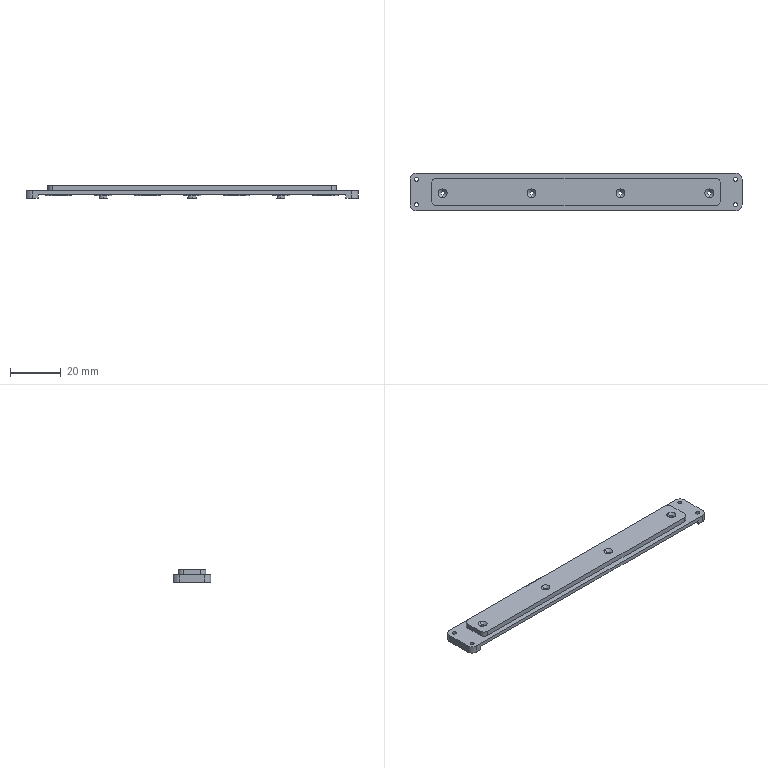NC program | NX | posted with a generic post | part box 130.666 x 14.95 x 5 mm
Lines 1 to 1700 of 3855:
N10 G17 G21 G94 G90
(FLOOR_WALL_COPY_COPY , TOOL : D80)
N12 T19 M6
N14 G54
N16 G17 G0 G90 X110.333 Y0. S6500 M3
N18 G43 Z30. H19
N20 Z5.5
N22 G94 G1 Z2.5 F1500.
N24 X105.333
N26 X-105.333
N28 X-110.333
N30 Z5.5
N32 G0 Z30.
N34 X110.333
N36 Z5.
N38 G1 Z2.
N40 X105.333
N42 X-105.333
N44 X-110.333
N46 Z5.
N48 G0 Z30.
N50 X110.333
N52 Z4.5
N54 G1 Z1.5
N56 X105.333
N58 X-105.333
N60 X-110.333
N62 Z4.5
N64 G0 Z30.
N66 X110.333
N68 Z4.
N70 G1 Z1.
N72 X105.333
N74 X-105.333
N76 X-110.333
N78 Z4.
N80 G0 Z30.
N82 X110.333
N84 Z3.5
N86 G1 Z0.5
N88 X105.333
N90 X-105.333
N92 X-110.333
N94 Z3.5
N96 G0 Z30.
N98 X110.333
N100 Z3.
N102 G1 Z0.
N104 X105.333
N106 X-105.333
N108 X-110.333
N110 Z3.
N112 G0 Z30.
N114 M5
(DRILLING_COPY_1_COPY_2 , TOOL : D6A45)
N116 T01 M6
N118 G54
N120 G17 G0 G90 X-34.994 Y0. S5000 M3
N122 G43 Z30. H1
N124 G94 G81 G98 Z-1.1 F350. R3.
N126 X0.006
N128 X35.006
N130 G80
N132 G0 X35.006 Y0. Z30.
N134 M5
(DRILLING_COPY_1_COPY_COPY_COPY , TOOL : 1.6ZT)
N136 T17 M6
N138 G54
N140 G17 G0 G90 X-34.994 Y0. S2000 M3
N142 G43 Z30. H17
N144 G94 G83 G98 Z-3.5 F100. Q2. R3.
N146 X35.006
N148 X0.006
N150 G80
N152 G0 X0.006 Y0. Z30.
N154 M5
(CAVITY_MILL , TOOL : D10)
N156 T15 M6
N158 G54
N160 G17 G0 G90 X-17.283 Y-14.473 S9500 M3
N162 G43 Z30. H15
N164 Z0.1
N166 G94 G1 Z-0.9 F1000.
N168 Y-8.02
N170 G3 X-17.494 Y-7.973 R0.5
N172 G1 Y-1.973
N174 X-7.644 F2500.
N176 G2 X-7.644 Y1.973 R7.9
N178 G1 X-6.482 Y1.673
N180 G2 X1.679 Y6.488 R6.7
N182 X-6.482 Y1.673 R-6.7
N184 G1 X-7.644 Y1.973
N186 X-27.345
N188 G2 X-27.345 Y-1.973 R7.9
N190 G1 X-28.507 Y-1.673
N192 G2 X-36.668 Y-6.488 R6.7
N194 X-28.507 Y-1.673 R-6.7
N196 G1 X-27.345 Y-1.973
N198 X-17.494
N200 Y-7.973
N202 X7.655
N204 Y-1.973
N206 X27.356
N208 G2 X27.356 Y1.973 R7.9
N210 G1 X28.518 Y1.673
N212 G2 X36.679 Y6.488 R6.7
N214 X28.518 Y1.673 R-6.7
N216 G1 X27.356 Y1.973
N218 X7.655
N220 G2 X7.655 Y-1.973 R7.9
N222 G1 Y-7.973
N224 X42.655
N226 Y-1.973
N228 X49.406
N230 Y1.973
N232 X42.655
N234 G2 X42.655 Y-1.973 R7.9
N236 G1 Y-7.973
N238 X54.225
N240 G3 X56.67 Y-12.473 R6.3
N242 G1 X59.491
N244 G2 X55.406 Y-7.475 R5.1
N246 G1 Y7.475
N248 G2 X59.491 Y12.473 R5.1
N250 G1 X56.67
N252 G3 X54.225 Y7.973 R6.3
N254 G1 X-42.644
N256 Y1.973
N258 X-49.394
N260 Y-1.973
N262 X-42.644
N264 G2 X-42.644 Y1.973 R7.9
N266 G1 Y7.973
N268 X-54.214
N270 G3 X-56.659 Y12.473 R6.3
N272 G1 X-59.479
N274 G2 X-55.394 Y7.475 R5.1
N276 G1 Y-7.475
N278 G2 X-59.479 Y-12.473 R5.1
N280 G1 X-56.659
N282 G3 X-54.214 Y-7.973 R6.3
N284 G1 X-17.494
N286 G2 X-16.728 Y-8.33 R1.
N288 G1 X-11.574 Y-14.473
N290 Z0.1
N292 G0 X-2.139 Z-0.4
N294 G1 Z-1.4 F1000.
N296 X-0.76 Y-12.83
N298 G2 X0.006 Y-12.473 R1.
N300 G1 X59.492 F2500.
N302 G2 X56.374 Y-10.464 R5.1
N304 X55.081 Y-10.575 R7.6
N306 G1 X49.931
N308 G2 X42.448 Y-4.31 R7.601
N310 X27.563 Y-4.309 R8.6
N312 X20.081 Y-10.575 R7.6
N314 G1 X14.931
N316 G2 X7.449 Y-4.309 R7.6
N318 X-7.437 Y-4.309 R8.6
N320 X-14.919 Y-10.575 R7.6
N322 G1 X-20.069
N324 G2 X-27.551 Y-4.309 R7.6
N326 X-42.437 Y-4.309 R8.6
N328 X-49.919 Y-10.575 R7.6
N330 G1 X-55.069
N332 G2 X-56.362 Y-10.464 R7.6
N334 X-59.481 Y-12.473 R5.1
N336 G1 X0.006
N338 G2 X0.772 Y-12.83 R1.
N340 G1 X2.15 Y-14.473
N342 Z-0.4
N344 G0 Z30.
N346 Y14.473
N348 Z-0.4
N350 G1 Z-1.4 F1000.
N352 X0.772 Y12.83
N354 G2 X0.006 Y12.473 R1.
N356 G1 X-59.481 F2500.
N358 G2 X-56.362 Y10.464 R5.1
N360 X-55.069 Y10.575 R7.6
N362 G1 X-49.919
N364 G2 X-42.436 Y4.31 R7.601
N366 X-27.551 Y4.309 R8.6
N368 X-20.069 Y10.575 R7.6
N370 G1 X-14.919
N372 G2 X-7.437 Y4.309 R7.6
N374 X7.449 Y4.309 R8.6
N376 X14.931 Y10.575 R7.6
N378 G1 X20.081
N380 G2 X27.563 Y4.309 R7.6
N382 X42.449 Y4.31 R8.601
N384 X49.931 Y10.575 R7.6
N386 G1 X55.081
N388 G2 X56.374 Y10.464 R7.6
N390 X59.492 Y12.473 R5.1
N392 G1 X0.006
N394 G2 X-0.76 Y12.83 R1.
N396 G1 X-2.139 Y14.473
N398 Z-0.4
N400 G0 Z30.
N402 M5
(CAVITY_MILL_COPY , TOOL : D4)
N404 T11 M6
N406 G54
N408 G17 G0 G90 X59.073 Y-9.881 S9500 M3
N410 G43 Z30. H11
N412 Z-0.25
N414 G94 G1 Z-1.25 F1000.
N416 X59.141 Y-9.544
N418 G3 X58.942 Y-8.722 R1.
N420 G2 X58.506 Y-7.475 R2. F1500.
N422 G1 Y-5.894
N424 G2 X55.851 Y-7.409 R4.5
N426 G3 X55.157 Y-7.892 R1.
N428 G1 X54.935 Y-8.275
N430 Z-0.25
N432 G0 X59.073 Y-9.881 Z-0.5
N434 G1 Z-1.5 F1000.
N436 X59.141 Y-9.544
N438 G3 X58.942 Y-8.722 R1.
N440 G2 X58.506 Y-7.475 R2. F1500.
N442 G1 Y-5.894
N444 G2 X55.851 Y-7.409 R4.5
N446 G3 X55.157 Y-7.892 R1.
N448 G1 X54.935 Y-8.275
N450 Z-0.5
N452 G0 Z30.
N454 Y8.275
N456 Z-0.25
N458 G1 Z-1.25 F1000.
N460 X55.157 Y7.892
N462 G3 X55.851 Y7.409 R1.
N464 G2 X58.506 Y5.894 R4.5 F1500.
N466 G1 Y7.475
N468 G2 X58.942 Y8.722 R2.
N470 G3 X59.141 Y9.544 R1.
N472 G1 X59.073 Y9.881
N474 Z-0.25
N476 G0 X54.935 Y8.275 Z-0.5
N478 G1 Z-1.5 F1000.
N480 X55.157 Y7.892
N482 G3 X55.851 Y7.409 R1.
N484 G2 X58.506 Y5.894 R4.5 F1500.
N486 G1 Y7.475
N488 G2 X58.942 Y8.722 R2.
N490 G3 X59.141 Y9.544 R1.
N492 G1 X59.073 Y9.881
N494 Z-0.5
N496 G0 Z30.
N498 X53.781 Y0.627
N500 Z1.5
N502 G1 Y1.675 Z1.445 F1000.
N504 X51.231 Z1.311
N506 Y-1.675 Z1.136
N508 X53.781 Z1.002
N510 Y1.675 Z0.827
N512 X51.231 Z0.693
N514 Y-1.675 Z0.517
N516 X53.781 Z0.384
N518 Y1.675 Z0.208
N520 X51.231 Z0.075
N522 Y-1.675 Z-0.101
N524 X53.781 Z-0.235
N526 Y1.675 Z-0.41
N528 X51.231 Z-0.544
N530 Y-1.675 Z-0.719
N532 X53.781 Z-0.853
N534 Y1.675 Z-1.029
N536 X51.231 Z-1.162
N538 Y0. Z-1.25
N540 Y-1.675 F1500.
N542 X53.781
N544 Y1.675
N546 X51.231
N548 Y0.
N550 G3 X51.588 Y-0.766 R1.
N552 G1 Z-0.25
N554 G0 X51.564 Y-1.675 Z0.25
N556 G1 X53.781 Z0.134 F1000.
N558 Y1.675 Z-0.042
N560 X51.231 Z-0.175
N562 Y-1.675 Z-0.351
N564 X53.781 Z-0.485
N566 Y1.675 Z-0.66
N568 X51.231 Z-0.794
N570 Y-1.675 Z-0.969
N572 X53.781 Z-1.103
N574 Y1.675 Z-1.279
N576 X51.231 Z-1.412
N578 Y0. Z-1.5
N580 Y-1.675 F1500.
N582 X53.781
N584 Y1.675
N586 X51.231
N588 Y0.
N590 G3 X51.588 Y-0.766 R1.
N592 G1 Z-0.5
N594 G0 X51.231 Y-1.054 Z0.
N596 G1 Y-1.675 Z-0.033 F1000.
N598 X53.781 Z-0.166
N600 Y1.675 Z-0.342
N602 X51.231 Z-0.475
N604 Y-1.675 Z-0.651
N606 X53.781 Z-0.785
N608 Y1.675 Z-0.96
N610 X51.231 Z-1.094
N612 Y-1.675 Z-1.269
N614 X53.781 Z-1.403
N616 Y1.675 Z-1.579
N618 X51.231 Z-1.712
N620 Y0. Z-1.8
N622 Y-1.675 F1500.
N624 X53.781
N626 Y1.675
N628 X51.231
N630 Y0.
N632 G3 X51.588 Y-0.766 R1.
N634 G1 Z-0.8
N636 G0 X51.231 Y-1.054 Z-0.3
N638 G1 Y-1.675 Z-0.333 F1000.
N640 X53.781 Z-0.466
N642 Y1.675 Z-0.642
N644 X51.231 Z-0.775
N646 Y-1.675 Z-0.951
N648 X53.781 Z-1.085
N650 Y1.675 Z-1.26
N652 X51.231 Z-1.394
N654 Y-1.675 Z-1.569
N656 X53.781 Z-1.703
N658 Y1.675 Z-1.879
N660 X51.231 Z-2.012
N662 Y0. Z-2.1
N664 Y-1.675 F1500.
N666 X53.781
N668 Y1.675
N670 X51.231
N672 Y0.
N674 G3 X51.588 Y-0.766 R1.
N676 G1 Z-1.1
N678 G0 X51.231 Y-1.054 Z-0.6
N680 G1 Y-1.675 Z-0.633 F1000.
N682 X53.781 Z-0.766
N684 Y1.675 Z-0.942
N686 X51.231 Z-1.075
N688 Y-1.675 Z-1.251
N690 X53.781 Z-1.385
N692 Y1.675 Z-1.56
N694 X51.231 Z-1.694
N696 Y-1.675 Z-1.869
N698 X53.781 Z-2.003
N700 Y1.675 Z-2.179
N702 X51.231 Z-2.312
N704 Y0. Z-2.4
N706 Y-1.675 F1500.
N708 X53.781
N710 Y1.675
N712 X51.231
N714 Y0.
N716 G3 X51.588 Y-0.766 R1.
N718 G1 Z-1.4
N720 G0 X51.231 Y-1.054 Z-0.9
N722 G1 Y-1.675 Z-0.933 F1000.
N724 X53.781 Z-1.066
N726 Y1.675 Z-1.242
N728 X51.231 Z-1.375
N730 Y-1.675 Z-1.551
N732 X53.781 Z-1.685
N734 Y1.675 Z-1.86
N736 X51.231 Z-1.994
N738 Y-1.675 Z-2.169
N740 X53.781 Z-2.303
N742 Y1.675 Z-2.479
N744 X51.231 Z-2.612
N746 Y0. Z-2.7
N748 Y-1.675 F1500.
N750 X53.781
N752 Y1.675
N754 X51.231
N756 Y0.
N758 G3 X51.588 Y-0.766 R1.
N760 G1 Z-1.7
N762 G0 Z30.
N764 X42.502 Y1.158
N766 Z-0.25
N768 G1 Z-1.25 F1000.
N770 X42.735 Y0.766
N772 G2 X43.092 Y0. R1.
N774 G3 X44.065 Y-1.98 R2.5 F1500.
N776 G2 X44.954 Y-3.272 R2.56
N778 G3 X45.478 Y-3.627 R0.5
N780 G2 X45.431 Y-2.975 R4.5
N782 G1 Y2.975
N784 G2 X45.478 Y3.627 R4.5
N786 G3 X44.954 Y3.272 R0.5
N788 G2 X44.065 Y1.98 R2.56
N790 G3 X43.092 Y0. R2.5
N792 G2 X42.735 Y-0.766 R1.
N794 G1 X42.502 Y-1.158
N796 Z-0.25
N798 G0 Y1.158 Z-0.5
N800 G1 Z-1.5 F1000.
N802 X42.735 Y0.766
N804 G2 X43.092 Y0. R1.
N806 G3 X44.065 Y-1.98 R2.5 F1500.
N808 G2 X44.954 Y-3.272 R2.56
N810 G3 X45.478 Y-3.627 R0.5
N812 G2 X45.431 Y-2.975 R4.5
N814 G1 Y2.975
N816 G2 X45.478 Y3.627 R4.5
N818 G3 X44.954 Y3.272 R0.5
N820 G2 X44.065 Y1.98 R2.56
N822 G3 X43.092 Y0. R2.5
N824 G2 X42.735 Y-0.766 R1.
N826 G1 X42.502 Y-1.158
N828 Z-0.5
N830 G0 Z30.
N832 X39.971 Y3.877
N834 Z-0.25
N836 G1 Z-1.25 F1000.
N838 X39.801 Y3.45
N840 G3 X39.849 Y2.606 R1.
N842 G2 X39.849 Y-2.606 R5.5 F1500.
N844 G3 X39.801 Y-3.45 R1.
N846 G1 X39.971 Y-3.877
N848 Z-0.25
N850 G0 Y3.877 Z-0.5
N852 G1 Z-1.5 F1000.
N854 X39.801 Y3.45
N856 G3 X39.849 Y2.606 R1.
N858 G2 X39.849 Y-2.606 R5.5 F1500.
N860 G3 X39.801 Y-3.45 R1.
N862 G1 X39.971 Y-3.877
N864 Z-0.5
N866 G0 Z30.
N868 X30.041 Y-3.878
N870 Z-0.25
N872 G1 Z-1.25 F1000.
N874 X30.211 Y-3.45
N876 G3 X30.163 Y-2.607 R1.
N878 G2 X30.164 Y2.609 R5.5 F1500.
N880 G3 X30.213 Y3.453 R1.
N882 G1 X30.043 Y3.881
N884 Z-0.25
N886 G0 X30.041 Y-3.878 Z-0.5
N888 G1 Z-1.5 F1000.
N890 X30.211 Y-3.45
N892 G3 X30.163 Y-2.607 R1.
N894 G2 X30.164 Y2.609 R5.5 F1500.
N896 G3 X30.213 Y3.453 R1.
N898 G1 X30.043 Y3.881
N900 Z-0.5
N902 G0 Z30.
N904 X27.51 Y-1.162
N906 Z-0.25
N908 G1 Z-1.25 F1000.
N910 X27.278 Y-0.766
N912 G2 X26.921 Y0. R1.
N914 G3 X25.947 Y1.98 R2.5 F1500.
N916 G2 X25.057 Y3.273 R2.56
N918 G3 X24.533 Y3.628 R0.5
N920 G2 X24.581 Y2.975 R4.5
N922 G1 Y-2.975
N924 G2 X24.533 Y-3.63 R4.5
N926 G3 X25.057 Y-3.275 R0.5
N928 G2 X25.947 Y-1.98 R2.56
N930 G3 X26.921 Y0. R2.5
N932 G2 X27.278 Y0.766 R1.
N934 G1 X27.51 Y1.163
N936 Z-0.25
N938 G0 Y-1.162 Z-0.5
N940 G1 Z-1.5 F1000.
N942 X27.278 Y-0.766
N944 G2 X26.921 Y0. R1.
N946 G3 X25.947 Y1.98 R2.5 F1500.
N948 G2 X25.057 Y3.273 R2.56
N950 G3 X24.533 Y3.628 R0.5
N952 G2 X24.581 Y2.975 R4.5
N954 G1 Y-2.975
N956 G2 X24.533 Y-3.63 R4.5
N958 G3 X25.057 Y-3.275 R0.5
N960 G2 X25.947 Y-1.98 R2.56
N962 G3 X26.921 Y0. R2.5
N964 G2 X27.278 Y0.766 R1.
N966 G1 X27.51 Y1.163
N968 Z-0.5
N970 G0 Z30.
N972 X18.781 Y0.627
N974 Z1.5
N976 G1 Y1.675 Z1.445 F1000.
N978 X16.231 Z1.311
N980 Y-1.675 Z1.136
N982 X18.781 Z1.002
N984 Y1.675 Z0.827
N986 X16.231 Z0.693
N988 Y-1.675 Z0.517
N990 X18.781 Z0.384
N992 Y1.675 Z0.208
N994 X16.231 Z0.075
N996 Y-1.675 Z-0.101
N998 X18.781 Z-0.235
N1000 Y1.675 Z-0.41
N1002 X16.231 Z-0.544
N1004 Y-1.675 Z-0.719
N1006 X18.781 Z-0.853
N1008 Y1.675 Z-1.029
N1010 X16.231 Z-1.162
N1012 Y0. Z-1.25
N1014 Y-1.675 F1500.
N1016 X18.781
N1018 Y1.675
N1020 X16.231
N1022 Y0.
N1024 G3 X16.588 Y-0.766 R1.
N1026 G1 Z-0.25
N1028 G0 X16.564 Y-1.675 Z0.25
N1030 G1 X18.781 Z0.134 F1000.
N1032 Y1.675 Z-0.042
N1034 X16.231 Z-0.175
N1036 Y-1.675 Z-0.351
N1038 X18.781 Z-0.485
N1040 Y1.675 Z-0.66
N1042 X16.231 Z-0.794
N1044 Y-1.675 Z-0.969
N1046 X18.781 Z-1.103
N1048 Y1.675 Z-1.279
N1050 X16.231 Z-1.412
N1052 Y0. Z-1.5
N1054 Y-1.675 F1500.
N1056 X18.781
N1058 Y1.675
N1060 X16.231
N1062 Y0.
N1064 G3 X16.588 Y-0.766 R1.
N1066 G1 Z-0.5
N1068 G0 X16.231 Y-1.054 Z0.
N1070 G1 Y-1.675 Z-0.033 F1000.
N1072 X18.781 Z-0.166
N1074 Y1.675 Z-0.342
N1076 X16.231 Z-0.475
N1078 Y-1.675 Z-0.651
N1080 X18.781 Z-0.785
N1082 Y1.675 Z-0.96
N1084 X16.231 Z-1.094
N1086 Y-1.675 Z-1.269
N1088 X18.781 Z-1.403
N1090 Y1.675 Z-1.579
N1092 X16.231 Z-1.712
N1094 Y0. Z-1.8
N1096 Y-1.675 F1500.
N1098 X18.781
N1100 Y1.675
N1102 X16.231
N1104 Y0.
N1106 G3 X16.588 Y-0.766 R1.
N1108 G1 Z-0.8
N1110 G0 X16.231 Y-1.054 Z-0.3
N1112 G1 Y-1.675 Z-0.333 F1000.
N1114 X18.781 Z-0.466
N1116 Y1.675 Z-0.642
N1118 X16.231 Z-0.775
N1120 Y-1.675 Z-0.951
N1122 X18.781 Z-1.085
N1124 Y1.675 Z-1.26
N1126 X16.231 Z-1.394
N1128 Y-1.675 Z-1.569
N1130 X18.781 Z-1.703
N1132 Y1.675 Z-1.879
N1134 X16.231 Z-2.012
N1136 Y0. Z-2.1
N1138 Y-1.675 F1500.
N1140 X18.781
N1142 Y1.675
N1144 X16.231
N1146 Y0.
N1148 G3 X16.588 Y-0.766 R1.
N1150 G1 Z-1.1
N1152 G0 X16.231 Y-1.054 Z-0.6
N1154 G1 Y-1.675 Z-0.633 F1000.
N1156 X18.781 Z-0.766
N1158 Y1.675 Z-0.942
N1160 X16.231 Z-1.075
N1162 Y-1.675 Z-1.251
N1164 X18.781 Z-1.385
N1166 Y1.675 Z-1.56
N1168 X16.231 Z-1.694
N1170 Y-1.675 Z-1.869
N1172 X18.781 Z-2.003
N1174 Y1.675 Z-2.179
N1176 X16.231 Z-2.312
N1178 Y0. Z-2.4
N1180 Y-1.675 F1500.
N1182 X18.781
N1184 Y1.675
N1186 X16.231
N1188 Y0.
N1190 G3 X16.588 Y-0.766 R1.
N1192 G1 Z-1.4
N1194 G0 X16.231 Y-1.054 Z-0.9
N1196 G1 Y-1.675 Z-0.933 F1000.
N1198 X18.781 Z-1.066
N1200 Y1.675 Z-1.242
N1202 X16.231 Z-1.375
N1204 Y-1.675 Z-1.551
N1206 X18.781 Z-1.685
N1208 Y1.675 Z-1.86
N1210 X16.231 Z-1.994
N1212 Y-1.675 Z-2.169
N1214 X18.781 Z-2.303
N1216 Y1.675 Z-2.479
N1218 X16.231 Z-2.612
N1220 Y0. Z-2.7
N1222 Y-1.675 F1500.
N1224 X18.781
N1226 Y1.675
N1228 X16.231
N1230 Y0.
N1232 G3 X16.588 Y-0.766 R1.
N1234 G1 Z-1.7
N1236 G0 Z30.
N1238 X7.502 Y1.158
N1240 Z-0.25
N1242 G1 Z-1.25 F1000.
N1244 X7.735 Y0.766
N1246 G2 X8.092 Y0. R1.
N1248 G3 X9.065 Y-1.98 R2.5 F1500.
N1250 G2 X9.954 Y-3.272 R2.56
N1252 G3 X10.478 Y-3.627 R0.5
N1254 G2 X10.431 Y-2.975 R4.5
N1256 G1 Y2.975
N1258 G2 X10.478 Y3.627 R4.5
N1260 G3 X9.954 Y3.272 R0.5
N1262 G2 X9.065 Y1.98 R2.56
N1264 G3 X8.092 Y0. R2.5
N1266 G2 X7.735 Y-0.766 R1.
N1268 G1 X7.502 Y-1.158
N1270 Z-0.25
N1272 G0 Y1.158 Z-0.5
N1274 G1 Z-1.5 F1000.
N1276 X7.735 Y0.766
N1278 G2 X8.092 Y0. R1.
N1280 G3 X9.065 Y-1.98 R2.5 F1500.
N1282 G2 X9.954 Y-3.272 R2.56
N1284 G3 X10.478 Y-3.627 R0.5
N1286 G2 X10.431 Y-2.975 R4.5
N1288 G1 Y2.975
N1290 G2 X10.478 Y3.627 R4.5
N1292 G3 X9.954 Y3.272 R0.5
N1294 G2 X9.065 Y1.98 R2.56
N1296 G3 X8.092 Y0. R2.5
N1298 G2 X7.735 Y-0.766 R1.
N1300 G1 X7.502 Y-1.158
N1302 Z-0.5
N1304 G0 Z30.
N1306 X4.971 Y3.877
N1308 Z-0.25
N1310 G1 Z-1.25 F1000.
N1312 X4.801 Y3.45
N1314 G3 X4.849 Y2.606 R1.
N1316 G2 X4.849 Y-2.606 R5.5 F1500.
N1318 G3 X4.801 Y-3.45 R1.
N1320 G1 X4.971 Y-3.877
N1322 Z-0.25
N1324 G0 Y3.877 Z-0.5
N1326 G1 Z-1.5 F1000.
N1328 X4.801 Y3.45
N1330 G3 X4.849 Y2.606 R1.
N1332 G2 X4.849 Y-2.606 R5.5 F1500.
N1334 G3 X4.801 Y-3.45 R1.
N1336 G1 X4.971 Y-3.877
N1338 Z-0.5
N1340 G0 Z30.
N1342 X-4.96
N1344 Z-0.25
N1346 G1 Z-1.25 F1000.
N1348 X-4.789 Y-3.45
N1350 G3 X-4.838 Y-2.606 R1.
N1352 G2 X-4.838 Y2.606 R5.5 F1500.
N1354 G3 X-4.789 Y3.45 R1.
N1356 G1 X-4.96 Y3.877
N1358 Z-0.25
N1360 G0 Y-3.877 Z-0.5
N1362 G1 Z-1.5 F1000.
N1364 X-4.789 Y-3.45
N1366 G3 X-4.838 Y-2.606 R1.
N1368 G2 X-4.838 Y2.606 R5.5 F1500.
N1370 G3 X-4.789 Y3.45 R1.
N1372 G1 X-4.96 Y3.877
N1374 Z-0.5
N1376 G0 Z30.
N1378 X-7.491 Y-1.158
N1380 Z-0.25
N1382 G1 Z-1.25 F1000.
N1384 X-7.723 Y-0.766
N1386 G2 X-8.081 Y0. R1.
N1388 G3 X-9.054 Y1.98 R2.5 F1500.
N1390 G2 X-9.943 Y3.272 R2.56
N1392 G3 X-10.467 Y3.627 R0.5
N1394 G2 X-10.419 Y2.975 R4.5
N1396 G1 Y-2.975
N1398 G2 X-10.467 Y-3.627 R4.5
N1400 G3 X-9.943 Y-3.272 R0.5
N1402 G2 X-9.054 Y-1.98 R2.56
N1404 G3 X-8.081 Y0. R2.5
N1406 G2 X-7.723 Y0.766 R1.
N1408 G1 X-7.491 Y1.158
N1410 Z-0.25
N1412 G0 Y-1.158 Z-0.5
N1414 G1 Z-1.5 F1000.
N1416 X-7.723 Y-0.766
N1418 G2 X-8.081 Y0. R1.
N1420 G3 X-9.054 Y1.98 R2.5 F1500.
N1422 G2 X-9.943 Y3.272 R2.56
N1424 G3 X-10.467 Y3.627 R0.5
N1426 G2 X-10.419 Y2.975 R4.5
N1428 G1 Y-2.975
N1430 G2 X-10.467 Y-3.627 R4.5
N1432 G3 X-9.943 Y-3.272 R0.5
N1434 G2 X-9.054 Y-1.98 R2.56
N1436 G3 X-8.081 Y0. R2.5
N1438 G2 X-7.723 Y0.766 R1.
N1440 G1 X-7.491 Y1.158
N1442 Z-0.5
N1444 G0 Z30.
N1446 X-16.219 Y0.627
N1448 Z1.5
N1450 G1 Y1.675 Z1.445 F1000.
N1452 X-18.769 Z1.311
N1454 Y-1.675 Z1.136
N1456 X-16.219 Z1.002
N1458 Y1.675 Z0.827
N1460 X-18.769 Z0.693
N1462 Y-1.675 Z0.517
N1464 X-16.219 Z0.384
N1466 Y1.675 Z0.208
N1468 X-18.769 Z0.075
N1470 Y-1.675 Z-0.101
N1472 X-16.219 Z-0.235
N1474 Y1.675 Z-0.41
N1476 X-18.769 Z-0.544
N1478 Y-1.675 Z-0.719
N1480 X-16.219 Z-0.853
N1482 Y1.675 Z-1.029
N1484 X-18.769 Z-1.162
N1486 Y0. Z-1.25
N1488 Y-1.675 F1500.
N1490 X-16.219
N1492 Y1.675
N1494 X-18.769
N1496 Y0.
N1498 G3 X-18.412 Y-0.766 R1.
N1500 G1 Z-0.25
N1502 G0 X-18.436 Y-1.675 Z0.25
N1504 G1 X-16.219 Z0.134 F1000.
N1506 Y1.675 Z-0.042
N1508 X-18.769 Z-0.175
N1510 Y-1.675 Z-0.351
N1512 X-16.219 Z-0.485
N1514 Y1.675 Z-0.66
N1516 X-18.769 Z-0.794
N1518 Y-1.675 Z-0.969
N1520 X-16.219 Z-1.103
N1522 Y1.675 Z-1.279
N1524 X-18.769 Z-1.412
N1526 Y0. Z-1.5
N1528 Y-1.675 F1500.
N1530 X-16.219
N1532 Y1.675
N1534 X-18.769
N1536 Y0.
N1538 G3 X-18.412 Y-0.766 R1.
N1540 G1 Z-0.5
N1542 G0 X-18.769 Y-1.054 Z0.
N1544 G1 Y-1.675 Z-0.033 F1000.
N1546 X-16.219 Z-0.166
N1548 Y1.675 Z-0.342
N1550 X-18.769 Z-0.475
N1552 Y-1.675 Z-0.651
N1554 X-16.219 Z-0.785
N1556 Y1.675 Z-0.96
N1558 X-18.769 Z-1.094
N1560 Y-1.675 Z-1.269
N1562 X-16.219 Z-1.403
N1564 Y1.675 Z-1.579
N1566 X-18.769 Z-1.712
N1568 Y0. Z-1.8
N1570 Y-1.675 F1500.
N1572 X-16.219
N1574 Y1.675
N1576 X-18.769
N1578 Y0.
N1580 G3 X-18.412 Y-0.766 R1.
N1582 G1 Z-0.8
N1584 G0 X-18.769 Y-1.054 Z-0.3
N1586 G1 Y-1.675 Z-0.333 F1000.
N1588 X-16.219 Z-0.466
N1590 Y1.675 Z-0.642
N1592 X-18.769 Z-0.775
N1594 Y-1.675 Z-0.951
N1596 X-16.219 Z-1.085
N1598 Y1.675 Z-1.26
N1600 X-18.769 Z-1.394
N1602 Y-1.675 Z-1.569
N1604 X-16.219 Z-1.703
N1606 Y1.675 Z-1.879
N1608 X-18.769 Z-2.012
N1610 Y0. Z-2.1
N1612 Y-1.675 F1500.
N1614 X-16.219
N1616 Y1.675
N1618 X-18.769
N1620 Y0.
N1622 G3 X-18.412 Y-0.766 R1.
N1624 G1 Z-1.1
N1626 G0 X-18.769 Y-1.054 Z-0.6
N1628 G1 Y-1.675 Z-0.633 F1000.
N1630 X-16.219 Z-0.766
N1632 Y1.675 Z-0.942
N1634 X-18.769 Z-1.075
N1636 Y-1.675 Z-1.251
N1638 X-16.219 Z-1.385
N1640 Y1.675 Z-1.56
N1642 X-18.769 Z-1.694
N1644 Y-1.675 Z-1.869
N1646 X-16.219 Z-2.003
N1648 Y1.675 Z-2.179
N1650 X-18.769 Z-2.312
N1652 Y0. Z-2.4
N1654 Y-1.675 F1500.
N1656 X-16.219
N1658 Y1.675
N1660 X-18.769
N1662 Y0.
N1664 G3 X-18.412 Y-0.766 R1.
N1666 G1 Z-1.4
N1668 G0 X-18.769 Y-1.054 Z-0.9
N1670 G1 Y-1.675 Z-0.933 F1000.
N1672 X-16.219 Z-1.066
N1674 Y1.675 Z-1.242
N1676 X-18.769 Z-1.375
N1678 Y-1.675 Z-1.551
N1680 X-16.219 Z-1.685
N1682 Y1.675 Z-1.86
N1684 X-18.769 Z-1.994
N1686 Y-1.675 Z-2.169
N1688 X-16.219 Z-2.303
N1690 Y1.675 Z-2.479
N1692 X-18.769 Z-2.612
N1694 Y0. Z-2.7
N1696 Y-1.675 F1500.
N1698 X-16.219
N1700 Y1.675
N1702 X-18.769
N1704 Y0.
N1706 G3 X-18.412 Y-0.766 R1.
N1708 G1 Z-1.7
N1710 G0 Z30.
N1712 X-27.498 Y1.158
N1714 Z-0.25
N1716 G1 Z-1.25 F1000.
N1718 X-27.265 Y0.766
N1720 G2 X-26.908 Y0. R1.
N1722 G3 X-25.935 Y-1.98 R2.5 F1500.
N1724 G2 X-25.046 Y-3.272 R2.56
N1726 G3 X-24.522 Y-3.627 R0.5
N1728 G2 X-24.569 Y-2.975 R4.5
N1730 G1 Y2.975
N1732 G2 X-24.522 Y3.627 R4.5
N1734 G3 X-25.046 Y3.272 R0.5
N1736 G2 X-25.935 Y1.98 R2.56
N1738 G3 X-26.908 Y0. R2.5
N1740 G2 X-27.265 Y-0.766 R1.
N1742 G1 X-27.498 Y-1.158
N1744 Z-0.25
N1746 G0 Y1.158 Z-0.5
N1748 G1 Z-1.5 F1000.
N1750 X-27.265 Y0.766
N1752 G2 X-26.908 Y0. R1.
N1754 G3 X-25.935 Y-1.98 R2.5 F1500.
N1756 G2 X-25.046 Y-3.272 R2.56
N1758 G3 X-24.522 Y-3.627 R0.5
N1760 G2 X-24.569 Y-2.975 R4.5
N1762 G1 Y2.975
N1764 G2 X-24.522 Y3.627 R4.5
N1766 G3 X-25.046 Y3.272 R0.5
N1768 G2 X-25.935 Y1.98 R2.56
N1770 G3 X-26.908 Y0. R2.5
N1772 G2 X-27.265 Y-0.766 R1.
N1774 G1 X-27.498 Y-1.158
N1776 Z-0.5
N1778 G0 Z30.
N1780 X-30.029 Y3.877
N1782 Z-0.25
N1784 G1 Z-1.25 F1000.
N1786 X-30.199 Y3.45
N1788 G3 X-30.151 Y2.606 R1.
N1790 G2 X-30.151 Y-2.606 R5.5 F1500.
N1792 G3 X-30.199 Y-3.45 R1.
N1794 G1 X-30.029 Y-3.877
N1796 Z-0.25
N1798 G0 Y3.877 Z-0.5
N1800 G1 Z-1.5 F1000.
N1802 X-30.199 Y3.45
N1804 G3 X-30.151 Y2.606 R1.
N1806 G2 X-30.151 Y-2.606 R5.5 F1500.
N1808 G3 X-30.199 Y-3.45 R1.
N1810 G1 X-30.029 Y-3.877
N1812 Z-0.5
N1814 G0 Z30.
N1816 X-39.96
N1818 Z-0.25
N1820 G1 Z-1.25 F1000.
N1822 X-39.789 Y-3.45
N1824 G3 X-39.838 Y-2.606 R1.
N1826 G2 X-39.823 Y2.633 R5.5 F1500.
N1828 G3 X-39.77 Y3.476 R1.
N1830 G1 X-39.938 Y3.905
N1832 Z-0.25
N1834 G0 X-39.96 Y-3.877 Z-0.5
N1836 G1 Z-1.5 F1000.
N1838 X-39.789 Y-3.45
N1840 G3 X-39.838 Y-2.606 R1.
N1842 G2 X-39.823 Y2.633 R5.5 F1500.
N1844 G3 X-39.77 Y3.476 R1.
N1846 G1 X-39.938 Y3.905
N1848 Z-0.5
N1850 G0 Z30.
N1852 X-42.491 Y-1.171
N1854 Z-0.25
N1856 G1 Z-1.25 F1000.
N1858 X-42.717 Y-0.761
N1860 G2 X-43.075 Y0.005 R1.
N1862 G3 X-44.052 Y1.987 R2.5 F1500.
N1864 G2 X-44.943 Y3.279 R2.56
N1866 G3 X-45.468 Y3.633 R0.5
N1868 G2 X-45.419 Y2.975 R4.5
N1870 G1 Y-2.975
N1872 G2 X-45.467 Y-3.627 R4.5
N1874 G3 X-44.943 Y-3.272 R0.5
N1876 G2 X-44.051 Y-1.977 R2.56
N1878 G3 X-43.075 Y0.005 R2.5
N1880 G2 X-42.718 Y0.771 R1.
N1882 G1 X-42.491 Y1.181
N1884 Z-0.25
N1886 G0 Y-1.171 Z-0.5
N1888 G1 Z-1.5 F1000.
N1890 X-42.717 Y-0.761
N1892 G2 X-43.075 Y0.005 R1.
N1894 G3 X-44.052 Y1.987 R2.5 F1500.
N1896 G2 X-44.943 Y3.279 R2.56
N1898 G3 X-45.468 Y3.633 R0.5
N1900 G2 X-45.419 Y2.975 R4.5
N1902 G1 Y-2.975
N1904 G2 X-45.467 Y-3.627 R4.5
N1906 G3 X-44.943 Y-3.272 R0.5
N1908 G2 X-44.051 Y-1.977 R2.56
N1910 G3 X-43.075 Y0.005 R2.5
N1912 G2 X-42.718 Y0.771 R1.
N1914 G1 X-42.491 Y1.181
N1916 Z-0.5
N1918 G0 Z30.
N1920 X-51.219 Y0.626
N1922 Z1.5
N1924 G1 Y1.675 Z1.445 F1000.
N1926 X-53.769 Z1.311
N1928 Y-1.675 Z1.136
N1930 X-51.219 Z1.002
N1932 Y1.675 Z0.827
N1934 X-53.769 Z0.693
N1936 Y-1.675 Z0.517
N1938 X-51.219 Z0.384
N1940 Y1.675 Z0.208
N1942 X-53.769 Z0.075
N1944 Y-1.675 Z-0.101
N1946 X-51.219 Z-0.235
N1948 Y1.675 Z-0.41
N1950 X-53.769 Z-0.544
N1952 Y-1.675 Z-0.719
N1954 X-51.219 Z-0.853
N1956 Y1.675 Z-1.029
N1958 X-53.769 Z-1.162
N1960 Y0. Z-1.25
N1962 Y-1.675 F1500.
N1964 X-51.219
N1966 Y1.675
N1968 X-53.769
N1970 Y0.
N1972 G3 X-53.412 Y-0.766 R1.
N1974 G1 Z-0.25
N1976 G0 X-53.437 Y-1.675 Z0.25
N1978 G1 X-51.219 Z0.134 F1000.
N1980 X-51.22 Y1.675 Z-0.042
N1982 X-53.769 Z-0.175
N1984 Y-1.675 Z-0.351
N1986 X-51.219 Z-0.485
N1988 X-51.22 Y1.675 Z-0.66
N1990 X-53.769 Z-0.794
N1992 Y-1.675 Z-0.969
N1994 X-51.219 Z-1.103
N1996 X-51.22 Y1.675 Z-1.279
N1998 X-53.769 Z-1.412
N2000 Y0. Z-1.5
N2002 Y-1.675 F1500.
N2004 X-51.219
N2006 X-51.22 Y1.675
N2008 X-53.769
N2010 Y0.
N2012 G3 X-53.412 Y-0.766 R1.
N2014 G1 Z-0.5
N2016 G0 X-53.769 Y-1.053 Z0.
N2018 G1 Y-1.675 Z-0.033 F1000.
N2020 X-51.219 Z-0.166
N2022 X-51.22 Y1.675 Z-0.342
N2024 X-53.769 Z-0.475
N2026 Y-1.675 Z-0.651
N2028 X-51.219 Z-0.785
N2030 X-51.22 Y1.675 Z-0.96
N2032 X-53.769 Z-1.094
N2034 Y-1.675 Z-1.269
N2036 X-51.219 Z-1.403
N2038 X-51.22 Y1.675 Z-1.579
N2040 X-53.769 Z-1.712
N2042 Y0. Z-1.8
N2044 Y-1.675 F1500.
N2046 X-51.219
N2048 X-51.22 Y1.675
N2050 X-53.769
N2052 Y0.
N2054 G3 X-53.412 Y-0.766 R1.
N2056 G1 Z-0.8
N2058 G0 X-53.769 Y-1.052 Z-0.3
N2060 G1 Y-1.675 Z-0.333 F1000.
N2062 X-51.219 Z-0.466
N2064 X-51.22 Y1.675 Z-0.642
N2066 X-53.769 Z-0.775
N2068 Y-1.675 Z-0.951
N2070 X-51.219 Z-1.085
N2072 X-51.22 Y1.675 Z-1.26
N2074 X-53.769 Z-1.394
N2076 Y-1.675 Z-1.569
N2078 X-51.219 Z-1.703
N2080 X-51.22 Y1.675 Z-1.879
N2082 X-53.769 Z-2.012
N2084 Y0. Z-2.1
N2086 Y-1.675 F1500.
N2088 X-51.219
N2090 X-51.22 Y1.675
N2092 X-53.769
N2094 Y0.
N2096 G3 X-53.412 Y-0.766 R1.
N2098 G1 Z-1.1
N2100 G0 X-53.769 Y-1.051 Z-0.6
N2102 G1 Y-1.675 Z-0.633 F1000.
N2104 X-51.219 Z-0.766
N2106 X-51.221 Y1.675 Z-0.942
N2108 X-53.769 Z-1.075
N2110 Y-1.675 Z-1.251
N2112 X-51.219 Z-1.385
N2114 X-51.221 Y1.675 Z-1.56
N2116 X-53.769 Z-1.694
N2118 Y-1.675 Z-1.869
N2120 X-51.219 Z-2.003
N2122 X-51.221 Y1.675 Z-2.179
N2124 X-53.769 Z-2.312
N2126 Y0. Z-2.4
N2128 Y-1.675 F1500.
N2130 X-51.219
N2132 X-51.221 Y1.675
N2134 X-53.769
N2136 Y0.
N2138 G3 X-53.412 Y-0.766 R1.
N2140 G1 Z-1.4
N2142 G0 X-53.769 Y-1.051 Z-0.9
N2144 G1 Y-1.675 Z-0.933 F1000.
N2146 X-51.219 Z-1.066
N2148 X-51.221 Y1.675 Z-1.242
N2150 X-53.769 Z-1.376
N2152 Y-1.675 Z-1.551
N2154 X-51.219 Z-1.685
N2156 X-51.221 Y1.675 Z-1.86
N2158 X-53.769 Z-1.994
N2160 Y-1.675 Z-2.169
N2162 X-51.219 Z-2.303
N2164 X-51.221 Y1.675 Z-2.479
N2166 X-53.769 Z-2.612
N2168 Y0. Z-2.7
N2170 Y-1.675 F1500.
N2172 X-51.219
N2174 X-51.221 Y1.675
N2176 X-53.769
N2178 Y0.
N2180 G3 X-53.412 Y-0.766 R1.
N2182 G1 Z-1.7
N2184 G0 Z30.
N2186 X-54.923 Y-8.275
N2188 Z-0.25
N2190 G1 Z-1.25 F1000.
N2192 X-55.146 Y-7.892
N2194 G3 X-55.839 Y-7.409 R1.
N2196 G2 X-58.494 Y-5.894 R4.5 F1500.
N2198 G1 Y-7.475
N2200 G2 X-58.931 Y-8.722 R2.
N2202 G3 X-59.129 Y-9.544 R1.
N2204 G1 X-59.061 Y-9.881
N2206 Z-0.25
N2208 G0 X-54.923 Y-8.275 Z-0.5
N2210 G1 Z-1.5 F1000.
N2212 X-55.146 Y-7.892
N2214 G3 X-55.839 Y-7.409 R1.
N2216 G2 X-58.494 Y-5.894 R4.5 F1500.
N2218 G1 Y-7.475
N2220 G2 X-58.931 Y-8.722 R2.
N2222 G3 X-59.129 Y-9.544 R1.
N2224 G1 X-59.061 Y-9.881
N2226 Z-0.5
N2228 G0 Z30.
N2230 Y9.881
N2232 Z-0.25
N2234 G1 Z-1.25 F1000.
N2236 X-59.129 Y9.544
N2238 G3 X-58.931 Y8.722 R1.
N2240 G2 X-58.494 Y7.475 R2. F1500.
N2242 G1 Y5.894
N2244 G2 X-55.839 Y7.409 R4.5
N2246 G3 X-55.146 Y7.892 R1.
N2248 G1 X-54.923 Y8.275
N2250 Z-0.25
N2252 G0 X-59.061 Y9.881 Z-0.5
N2254 G1 Z-1.5 F1000.
N2256 X-59.129 Y9.544
N2258 G3 X-58.931 Y8.722 R1.
N2260 G2 X-58.494 Y7.475 R2. F1500.
N2262 G1 Y5.894
N2264 G2 X-55.839 Y7.409 R4.5
N2266 G3 X-55.146 Y7.892 R1.
N2268 G1 X-54.923 Y8.275
N2270 Z-0.5
N2272 G0 Z30.
(FLOOR_WALL_COPY_1_COPY , TOOL : D4)
N2274 X-44.419 Y0.
N2276 Z0.
N2278 G1 Z-1. F1000.
N2280 X-45.419
N2282 Y-2.975 F1200.
N2284 G2 X-49.919 Y-7.475 R4.5
N2286 G1 X-55.069
N2288 G2 X-58.361 Y-6.043 R4.5
N2290 G1 X-58.284 Y-5.988
N2292 X-58.294 Y-5.894
N2294 Y5.894
N2296 X-58.284 Y5.988
N2298 X-58.361 Y6.043
N2300 G2 X-55.069 Y7.475 R4.5
N2302 G1 X-49.919
N2304 G2 X-45.419 Y2.975 R4.5
N2306 G1 Y0.
N2308 X-47.419
N2310 Y-2.975
N2312 G2 X-49.919 Y-5.475 R2.5
N2314 G1 X-55.069
N2316 G2 X-56.294 Y-5.154 R2.5
N2318 G1 Y5.154
N2320 G2 X-55.069 Y5.475 R2.5
N2322 G1 X-49.919
N2324 G2 X-47.419 Y2.975 R2.5
N2326 G1 Y0.
N2328 X-49.419
N2330 Y-2.975
N2332 G2 X-49.919 Y-3.475 R0.5
N2334 G1 X-54.294
N2336 Y3.475
N2338 X-49.919
N2340 G2 X-49.419 Y2.975 R0.5
N2342 G1 Y0.
N2344 X-51.419
N2346 Y-1.475
N2348 X-52.294
N2350 Y1.475
N2352 X-51.419
N2354 Y0.
N2356 X-50.419
N2358 Z0.
N2360 G0 Z30.
N2362 X-57.494 Y7.912
N2364 Z0.
N2366 G1 Z-1. F1000.
N2368 X-58.494 Y6.894
N2370 Y5.894
N2372 Y-5.894 F1200.
N2374 Y-6.894
N2376 X-57.494 Y-7.912
N2378 Z0.
N2380 G0 Z30.
N2382 X-53.569 Y0.995
N2384 Z-1.6
N2386 G1 Y1.475 Z-1.729 F1000.
N2388 X-51.419 Z-2.305
N2390 Y0. Z-2.7
N2392 Y-1.475 F1200.
N2394 X-53.569
N2396 Y1.475
N2398 X-51.419
N2400 Y0.
N2402 X-52.419
N2404 X-51.219 F1000.
N2406 Y1.675 F1200.
N2408 X-53.769
N2410 Y-1.675
N2412 X-51.219
N2414 Y0.
N2416 X-52.219
N2418 Z-1.7
N2420 G0 Z30.
N2422 X-34.994 Y4.8
N2424 Z0.
N2426 G1 Z-1. F1000.
N2428 Y3.8
N2430 G2 X-31.194 Y0. R3.8 F1200.
N2432 X-34.994 Y3.8 R-3.8
N2434 G1 Y6.5
N2436 Y3.6 F1000.
N2438 G2 X-31.394 Y0. R3.6 F1200.
N2440 X-34.994 Y3.6 R-3.6
N2442 G1 Y4.8
N2444 Z0.
N2446 G0 Z30.
N2448 X-17.494 Y8.475
N2450 Z0.
N2452 G1 Z-1. F1000.
N2454 Y7.475
N2456 X-14.919 F1200.
N2458 G2 X-10.419 Y2.975 R4.5
N2460 G1 Y-2.975
N2462 G2 X-14.919 Y-7.475 R4.5
N2464 G1 X-20.069
N2466 G2 X-24.569 Y-2.975 R4.5
N2468 G1 Y2.975
N2470 G2 X-20.069 Y7.475 R4.5
N2472 G1 X-17.494
N2474 Y5.475
N2476 X-14.919
N2478 G2 X-12.419 Y2.975 R2.5
N2480 G1 Y-2.975
N2482 G2 X-14.919 Y-5.475 R2.5
N2484 G1 X-20.069
N2486 G2 X-22.569 Y-2.975 R2.5
N2488 G1 Y2.975
N2490 G2 X-20.069 Y5.475 R2.5
N2492 G1 X-17.494
N2494 Y3.475
N2496 X-14.919
N2498 G2 X-14.419 Y2.975 R0.5
N2500 G1 Y-2.975
N2502 G2 X-14.919 Y-3.475 R0.5
N2504 G1 X-20.069
N2506 G2 X-20.569 Y-2.975 R0.5
N2508 G1 Y2.975
N2510 G2 X-20.069 Y3.475 R0.5
N2512 G1 X-17.494
N2514 Y1.475
N2516 X-16.419
N2518 Y-1.475
N2520 X-18.569
N2522 Y1.475
N2524 X-17.494
N2526 Y2.475
N2528 Z0.
N2530 G0 Z30.
N2532 X-16.419 Y-0.995
N2534 Z-1.6
N2536 G1 Y-1.475 Z-1.729 F1000.
N2538 X-18.569 Z-2.305
N2540 Y0. Z-2.7
N2542 Y1.475 F1200.
N2544 X-16.419
N2546 Y-1.475
N2548 X-18.569
N2550 Y0.
N2552 X-17.569
N2554 X-18.769 F1000.
N2556 Y-1.675 F1200.
N2558 X-16.219
N2560 Y1.675
N2562 X-18.769
N2564 Y0.
N2566 X-17.769
N2568 Z-1.7
N2570 G0 Z30.
N2572 X0.006 Y4.8
N2574 Z0.
N2576 G1 Z-1. F1000.
N2578 Y3.8
N2580 G2 X3.806 Y0. R3.8 F1200.
N2582 X0.006 Y3.8 R-3.8
N2584 G1 Y6.5
N2586 Y3.6 F1000.
N2588 G2 X3.606 Y0. R3.6 F1200.
N2590 X0.006 Y3.6 R-3.6
N2592 G1 Y4.8
N2594 Z0.
N2596 G0 Z30.
N2598 X-5.479 Y10.475
N2600 Z-0.5
N2602 G1 Z-1.5 F1000.
N2604 Y9.475
N2606 X58.306 F1200.
N2608 Y6.394
N2610 G3 X55.081 Y7.675 R4.7
N2612 G1 X49.931
N2614 G3 X45.231 Y2.975 R4.7
N2616 G1 Y-2.975
N2618 G3 X49.931 Y-7.675 R4.7
N2620 G1 X55.081
N2622 G3 X58.306 Y-6.394 R4.7
N2624 G1 Y-9.475
N2626 X22.481
N2628 Y-7.475
N2630 G3 X25.181 Y-2.975 R5.1
N2632 G1 Y2.975
N2634 G3 X22.481 Y7.475 R5.1
N2636 G1 X44.967
N2638 G3 X43.231 Y2.975 R6.7
N2640 G1 Y-2.975
N2642 G3 X44.967 Y-7.475 R6.7
N2644 G1 X37.695
N2646 Y-5.475
N2648 G3 X37.695 Y5.475 R6.1
N2650 G1 X41.598
N2652 G3 X41.231 Y2.975 R8.7
N2654 G1 Y-2.975
N2656 G3 X41.598 Y-5.475 R8.7
N2658 G1 X37.695
N2660 Y-7.475
N2662 X22.481
N2664 X26.726 Y-5.475
N2666 G3 X27.181 Y-2.975 R7.1
N2668 G1 Y2.975
N2670 G3 X26.726 Y5.475 R7.1
N2672 G1 X32.316
N2674 G3 X32.316 Y-5.475 R6.1
N2676 G1 X32.492 Y-5.116
N2678 G2 X29.89 Y2.513 R5.7
N2680 X32.492 Y-5.116 R-5.7
N2682 G1 X32.316 Y-5.475
N2684 X26.726
N2686 X22.481 Y-7.475
N2688 Y-9.475
N2690 X-58.294
N2692 Y-6.394
N2694 G3 X-55.069 Y-7.675 R4.7
N2696 G1 X-49.919
N2698 G3 X-45.219 Y-2.975 R4.7
N2700 G1 Y2.975
N2702 G3 X-49.919 Y7.675 R4.7
N2704 G1 X-55.069
N2706 G3 X-58.294 Y6.394 R4.7
N2708 G1 Y9.475
N2710 X-22.469
N2712 Y7.475
N2714 G3 X-25.169 Y2.975 R5.1
N2716 G1 Y-2.975
N2718 G3 X-22.469 Y-7.475 R5.1
N2720 G1 X-44.955
N2722 G3 X-43.219 Y-2.975 R6.7
N2724 G1 Y2.975
N2726 G3 X-44.955 Y7.475 R6.7
N2728 G1 X-37.684
N2730 Y5.475
N2732 G3 X-37.684 Y-5.475 R6.1
N2734 G1 X-41.586
N2736 G3 X-41.219 Y-2.975 R8.7
N2738 G1 Y2.975
N2740 G3 X-41.586 Y5.475 R8.7
N2742 G1 X-37.684
N2744 Y7.475
N2746 X-22.469
N2748 X-26.715 Y5.475
N2750 G3 X-27.169 Y2.975 R7.1
N2752 G1 Y-2.975
N2754 G3 X-26.715 Y-5.475 R7.1
N2756 G1 X-32.305
N2758 G3 X-32.305 Y5.475 R6.1
N2760 G1 X-32.481 Y5.116
N2762 G2 X-29.878 Y-2.513 R5.7
N2764 X-32.481 Y5.116 R-5.7
N2766 G1 X-32.305 Y5.475
N2768 X-26.715
N2770 X-22.469 Y7.475
N2772 Y9.475
N2774 X-5.479
N2776 Y7.475
N2778 X12.531
N2780 G3 X9.831 Y2.975 R5.1
N2782 G1 Y-2.975
N2784 G3 X12.531 Y-7.475 R5.1
N2786 G1 X12.719 Y-7.122
N2788 G2 X10.231 Y-2.975 R4.7
N2790 G1 Y2.975
N2792 G2 X14.931 Y7.675 R4.7
N2794 G1 X20.081
N2796 G2 X24.781 Y2.975 R4.7
N2798 G1 Y-2.975
N2800 G2 X20.081 Y-7.675 R4.7
N2802 G1 X14.931
N2804 G2 X12.719 Y-7.122 R4.7
N2806 G1 X12.531 Y-7.475
N2808 X2.695
N2810 Y-5.475
N2812 G3 X2.695 Y5.475 R6.1
N2814 G1 X8.285
N2816 G3 X7.831 Y2.975 R7.1
N2818 G1 Y-2.975
N2820 G3 X8.285 Y-5.475 R7.1
N2822 G1 X2.695
N2824 Y-7.475
N2826 X-12.519
N2828 G3 X-9.819 Y-2.975 R5.1
N2830 G1 Y2.975
N2832 G3 X-12.519 Y7.475 R5.1
N2834 G1 X-12.707 Y7.122
N2836 G2 X-10.219 Y2.975 R4.7
N2838 G1 Y-2.975
N2840 G2 X-14.919 Y-7.675 R4.7
N2842 G1 X-20.069
N2844 G2 X-24.769 Y-2.975 R4.7
N2846 G1 Y2.975
N2848 G2 X-20.069 Y7.675 R4.7
N2850 G1 X-14.919
N2852 G2 X-12.707 Y7.122 R4.7
N2854 G1 X-12.519 Y7.475
N2856 X-5.479
N2858 Y5.475
N2860 X-2.684
N2862 G3 X-2.684 Y-5.475 R6.1
N2864 G1 X-2.508 Y-5.116
N2866 G2 X-5.11 Y2.513 R5.7
N2868 X-2.508 Y-5.116 R-5.7
N2870 G1 X-2.684 Y-5.475
N2872 X-8.274
N2874 G3 X-7.819 Y-2.975 R7.1
N2876 G1 Y2.975
N2878 G3 X-8.274 Y5.475 R7.1
N2880 G1 X-5.479
N2882 Y6.475
N2884 Z-0.5
N2886 G0 Z30.
N2888 X-58.494 Y10.475
N2890 Z-0.5
N2892 G1 Z-1.5 F1000.
N2894 Y9.475
N2896 Y5.894 F1200.
N2898 G2 X-55.069 Y7.475 R4.5
N2900 G1 X-49.919
N2902 G2 X-45.419 Y2.975 R4.5
N2904 G1 Y-2.975
N2906 G2 X-49.919 Y-7.475 R4.5
N2908 G1 X-55.069
N2910 G2 X-58.494 Y-5.894 R4.5
N2912 G1 Y-9.475
N2914 Y-10.475
N2916 Z-0.5
N2918 G0 Z30.
N2920 X58.506
N2922 Z-0.5
N2924 G1 Z-1.5 F1000.
N2926 Y-9.475
N2928 Y-5.894 F1200.
N2930 G2 X55.081 Y-7.475 R4.5
N2932 G1 X49.931
N2934 G2 X45.431 Y-2.975 R4.5
N2936 G1 Y2.975
N2938 G2 X49.931 Y7.475 R4.5
N2940 G1 X55.081
N2942 G2 X58.506 Y5.894 R4.5
N2944 G1 Y9.475
N2946 Y10.475
N2948 Z-0.5
N2950 G0 Z30.
N2952 X35.006 Y6.7
N2954 Z-0.5
N2956 G1 Z-1.5 F1000.
N2958 Y5.5
N2960 G2 X40.506 Y0. R5.5 F1200.
N2962 X35.006 Y5.5 R-5.5
N2964 G1 Y6.7
N2966 Z-0.5
N2968 G0 Z30.
N2970 X25.781 Y0.
N2972 Z-0.5
N2974 G1 Z-1.5 F1000.
N2976 X24.581
N2978 Y-2.975 F1200.
N2980 G2 X20.081 Y-7.475 R4.5
N2982 G1 X14.931
N2984 G2 X10.431 Y-2.975 R4.5
N2986 G1 Y2.975
N2988 G2 X14.931 Y7.475 R4.5
N2990 G1 X20.081
N2992 G2 X24.581 Y2.975 R4.5
N2994 G1 Y0.
N2996 X25.781
N2998 Z-0.5
N3000 G0 Z30.
N3002 X0.006 Y6.7
N3004 Z-0.5
N3006 G1 Z-1.5 F1000.
N3008 Y5.5
N3010 G2 X5.506 Y0. R5.5 F1200.
N3012 X0.006 Y5.5 R-5.5
N3014 G1 Y6.7
N3016 Z-0.5
N3018 G0 Z30.
N3020 X-9.219 Y0.
N3022 Z-0.5
N3024 G1 Z-1.5 F1000.
N3026 X-10.419
N3028 Y-2.975 F1200.
N3030 G2 X-14.919 Y-7.475 R4.5
N3032 G1 X-20.069
N3034 G2 X-24.569 Y-2.975 R4.5
N3036 G1 Y2.975
N3038 G2 X-20.069 Y7.475 R4.5
N3040 G1 X-14.919
N3042 G2 X-10.419 Y2.975 R4.5
N3044 G1 Y0.
N3046 X-9.219
N3048 Z-0.5
N3050 G0 Z30.
N3052 X-34.994 Y6.7
N3054 Z-0.5
N3056 G1 Z-1.5 F1000.
N3058 Y5.5
N3060 G2 X-29.494 Y0. R5.5 F1200.
N3062 X-34.994 Y5.5 R-5.5
N3064 G1 Y6.7
N3066 Z-0.5
N3068 G0 Z30.
N3070 X17.506 Y8.475
N3072 Z0.
N3074 G1 Z-1. F1000.
N3076 Y7.475
N3078 X20.081 F1200.
N3080 G2 X24.581 Y2.975 R4.5
N3082 G1 Y-2.975
N3084 G2 X20.081 Y-7.475 R4.5
N3086 G1 X14.931
N3088 G2 X10.431 Y-2.975 R4.5
N3090 G1 Y2.975
N3092 G2 X14.931 Y7.475 R4.5
N3094 G1 X17.506
N3096 Y5.475
N3098 X20.081
N3100 G2 X22.581 Y2.975 R2.5
N3102 G1 Y-2.975
N3104 G2 X20.081 Y-5.475 R2.5
N3106 G1 X14.931
N3108 G2 X12.431 Y-2.975 R2.5
N3110 G1 Y2.975
N3112 G2 X14.931 Y5.475 R2.5
N3114 G1 X17.506
N3116 Y3.475
N3118 X20.081
N3120 G2 X20.581 Y2.975 R0.5
N3122 G1 Y-2.975
N3124 G2 X20.081 Y-3.475 R0.5
N3126 G1 X14.931
N3128 G2 X14.431 Y-2.975 R0.5
N3130 G1 Y2.975
N3132 G2 X14.931 Y3.475 R0.5
N3134 G1 X17.506
N3136 Y1.475
N3138 X18.581
N3140 Y-1.475
N3142 X16.431
N3144 Y1.475
N3146 X17.506
N3148 Y2.475
N3150 Z0.
N3152 G0 Z30.
N3154 X16.431 Y0.995
N3156 Z-1.6
N3158 G1 Y1.475 Z-1.729 F1000.
N3160 X18.581 Z-2.305
N3162 Y0. Z-2.7
N3164 Y-1.475 F1200.
N3166 X16.431
N3168 Y1.475
N3170 X18.581
N3172 Y0.
N3174 X17.581
N3176 X18.781 F1000.
N3178 Y1.675 F1200.
N3180 X16.231
N3182 Y-1.675
N3184 X18.781
N3186 Y0.
N3188 X17.781
N3190 Z-1.7
N3192 G0 Z30.
N3194 X35.006 Y4.8
N3196 Z0.
N3198 G1 Z-1. F1000.
N3200 Y3.8
N3202 G2 X38.806 Y0. R3.8 F1200.
N3204 X35.006 Y3.8 R-3.8
N3206 G1 Y6.5
N3208 Y3.6 F1000.
N3210 G2 X38.606 Y0. R3.6 F1200.
N3212 X35.006 Y3.6 R-3.6
N3214 G1 Y4.8
N3216 Z0.
N3218 G0 Z30.
N3220 X44.431 Y0.
N3222 Z0.
N3224 G1 Z-1. F1000.
N3226 X45.431
N3228 Y2.975 F1200.
N3230 G2 X49.931 Y7.475 R4.5
N3232 G1 X55.081
N3234 G2 X58.373 Y6.043 R4.5
N3236 G1 X58.296 Y5.988
N3238 X58.306 Y5.894
N3240 Y-5.894
N3242 X58.296 Y-5.988
N3244 X58.373 Y-6.043
N3246 G2 X55.081 Y-7.475 R4.5
N3248 G1 X49.931
N3250 G2 X45.431 Y-2.975 R4.5
N3252 G1 Y0.
N3254 X47.431
N3256 Y2.975
N3258 G2 X49.931 Y5.475 R2.5
N3260 G1 X55.081
N3262 G2 X56.306 Y5.154 R2.5
N3264 G1 Y-5.154
N3266 G2 X55.081 Y-5.475 R2.5
N3268 G1 X49.931
N3270 G2 X47.431 Y-2.975 R2.5
N3272 G1 Y0.
N3274 X49.431
N3276 Y2.975
N3278 G2 X49.931 Y3.475 R0.5
N3280 G1 X54.306
N3282 Y-3.475
N3284 X49.931
N3286 G2 X49.431 Y-2.975 R0.5
N3288 G1 Y0.
N3290 X51.431
N3292 Y1.475
N3294 X52.306
N3296 Y-1.475
N3298 X51.431
N3300 Y0.
N3302 X50.431
N3304 Z0.
N3306 G0 Z30.
N3308 X57.506 Y-7.912
N3310 Z0.
N3312 G1 Z-1. F1000.
N3314 X58.506 Y-6.894
N3316 Y-5.894
N3318 Y5.894 F1200.
N3320 Y6.894
N3322 X57.506 Y7.912
N3324 Z0.
N3326 G0 Z30.
N3328 X53.581 Y-0.995
N3330 Z-1.6
N3332 G1 Y-1.475 Z-1.729 F1000.
N3334 X51.431 Z-2.305
N3336 Y0. Z-2.7
N3338 Y1.475 F1200.
N3340 X53.581
N3342 Y-1.475
N3344 X51.431
N3346 Y0.
N3348 X52.431
N3350 X51.231 F1000.
N3352 Y-1.675 F1200.
N3354 X53.781
N3356 Y1.675
N3358 X51.231
N3360 Y0.
N3362 X52.231
N3364 Z-1.7
N3366 G0 Z30.
N3368 M5